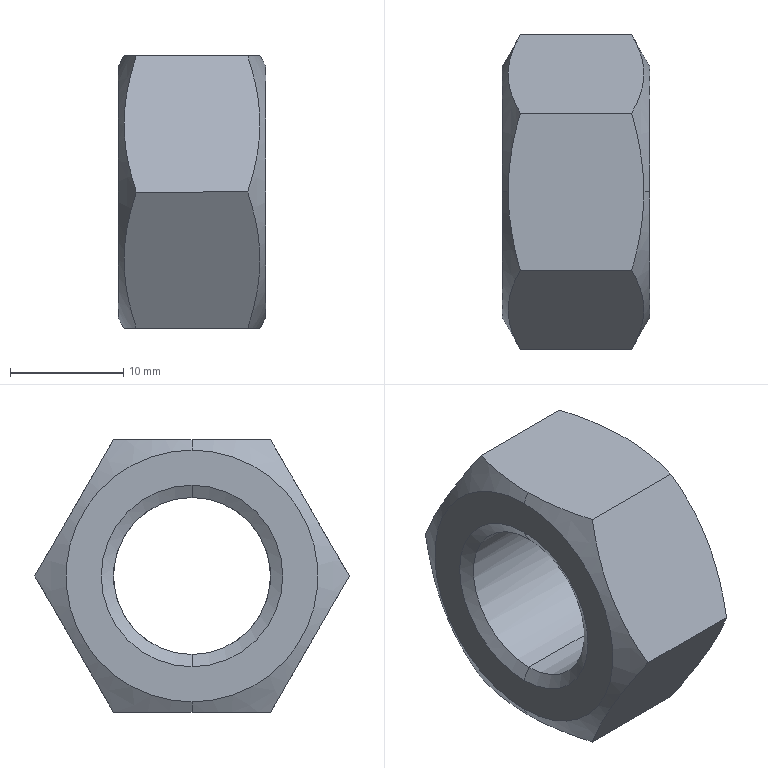Part | SolidWorks | features BaseBody 1 | 1 solid | 18 faces | box 13 x 27.713 x 24 mm | volume 4387 mm3 | cone 8 | plane 8 | cylinder 2 | commonest cylinder face diameters 13.835 x2
STEP:
#1=CARTESIAN_POINT('',(0.625,0.,6.918));
#2=VERTEX_POINT('',#1);
#3=CARTESIAN_POINT('',(0.625,0.,-6.918));
#4=VERTEX_POINT('',#3);
#5=CARTESIAN_POINT('',(0.625,0.,0.));
#6=DIRECTION('',(1.,0.,0.));
#7=DIRECTION('',(0.,0.,-1.));
#8=AXIS2_PLACEMENT_3D('',#5,#6,#7);
#9=CIRCLE('',#8,6.918);
#10=EDGE_CURVE('',#2,#4,#9,.T.);
#11=ORIENTED_EDGE('',*,*,#10,.F.);
#12=CARTESIAN_POINT('',(12.375,0.,6.918));
#13=VERTEX_POINT('',#12);
#14=CARTESIAN_POINT('',(-26.178,0.,6.918));
#15=DIRECTION('',(1.,0.,0.));
#16=VECTOR('',#15,1000.);
#17=LINE('',#14,#16);
#18=EDGE_CURVE('',#2,#13,#17,.T.);
#19=ORIENTED_EDGE('',*,*,#18,.T.);
#20=CARTESIAN_POINT('',(12.375,-6.918,0.));
#21=VERTEX_POINT('',#20);
#22=CARTESIAN_POINT('',(12.375,0.,0.));
#23=DIRECTION('',(-1.,0.,0.));
#24=DIRECTION('',(0.,0.,-1.));
#25=AXIS2_PLACEMENT_3D('',#22,#23,#24);
#26=CIRCLE('',#25,6.918);
#27=EDGE_CURVE('',#21,#13,#26,.T.);
#28=ORIENTED_EDGE('',*,*,#27,.F.);
#29=CARTESIAN_POINT('',(12.375,0.,-6.918));
#30=VERTEX_POINT('',#29);
#31=CARTESIAN_POINT('',(12.375,0.,0.));
#32=DIRECTION('',(-1.,0.,0.));
#33=DIRECTION('',(0.,0.,-1.));
#34=AXIS2_PLACEMENT_3D('',#31,#32,#33);
#35=CIRCLE('',#34,6.918);
#36=EDGE_CURVE('',#30,#21,#35,.T.);
#37=ORIENTED_EDGE('',*,*,#36,.F.);
#38=CARTESIAN_POINT('',(-26.178,0.,-6.918));
#39=DIRECTION('',(1.,0.,0.));
#40=VECTOR('',#39,1000.);
#41=LINE('',#38,#40);
#42=EDGE_CURVE('',#4,#30,#41,.T.);
#43=ORIENTED_EDGE('',*,*,#42,.F.);
#44=EDGE_LOOP('',(#11,#19,#28,#37,#43));
#45=FACE_OUTER_BOUND('',#44,.T.);
#46=CARTESIAN_POINT('',(-26.178,0.,0.));
#47=DIRECTION('',(1.,0.,0.));
#48=DIRECTION('',(0.,0.,-1.));
#49=AXIS2_PLACEMENT_3D('',#46,#47,#48);
#50=CYLINDRICAL_SURFACE('',#49,6.918);
#51=ADVANCED_FACE('',(#45),#50,.F.);
#52=ORIENTED_EDGE('',*,*,#10,.T.);
#53=CARTESIAN_POINT('',(0.,0.,-8.));
#54=VERTEX_POINT('',#53);
#55=CARTESIAN_POINT('',(0.,0.,-8.));
#56=DIRECTION('',(-0.5,0.,-0.866));
#57=VECTOR('',#56,1000.);
#58=LINE('',#55,#57);
#59=EDGE_CURVE('',#4,#54,#58,.T.);
#60=ORIENTED_EDGE('',*,*,#59,.T.);
#61=CARTESIAN_POINT('',(0.,0.,8.));
#62=VERTEX_POINT('',#61);
#63=CARTESIAN_POINT('',(0.,0.,0.));
#64=DIRECTION('',(1.,0.,0.));
#65=DIRECTION('',(0.,0.,1.));
#66=AXIS2_PLACEMENT_3D('',#63,#64,#65);
#67=CIRCLE('',#66,8.);
#68=EDGE_CURVE('',#62,#54,#67,.T.);
#69=ORIENTED_EDGE('',*,*,#68,.F.);
#70=CARTESIAN_POINT('',(0.,0.,8.));
#71=DIRECTION('',(-0.5,0.,0.866));
#72=VECTOR('',#71,1000.);
#73=LINE('',#70,#72);
#74=EDGE_CURVE('',#2,#62,#73,.T.);
#75=ORIENTED_EDGE('',*,*,#74,.F.);
#76=EDGE_LOOP('',(#52,#60,#69,#75));
#77=FACE_OUTER_BOUND('',#76,.T.);
#78=CARTESIAN_POINT('',(0.,0.,0.));
#79=DIRECTION('',(-1.,0.,0.));
#80=DIRECTION('',(0.,0.,1.));
#81=AXIS2_PLACEMENT_3D('',#78,#79,#80);
#82=CONICAL_SURFACE('',#81,8.,1.047);
#83=ADVANCED_FACE('',(#77),#82,.F.);
#84=CARTESIAN_POINT('',(12.375,6.918,0.));
#85=VERTEX_POINT('',#84);
#86=CARTESIAN_POINT('',(12.375,0.,0.));
#87=DIRECTION('',(-1.,0.,0.));
#88=DIRECTION('',(0.,0.,-1.));
#89=AXIS2_PLACEMENT_3D('',#86,#87,#88);
#90=CIRCLE('',#89,6.918);
#91=EDGE_CURVE('',#85,#30,#90,.T.);
#92=ORIENTED_EDGE('',*,*,#91,.T.);
#93=ORIENTED_EDGE('',*,*,#36,.T.);
#94=CARTESIAN_POINT('',(13.,-8.,0.));
#95=VERTEX_POINT('',#94);
#96=CARTESIAN_POINT('',(13.,-8.,0.));
#97=DIRECTION('',(0.5,-0.866,0.));
#98=VECTOR('',#97,1000.);
#99=LINE('',#96,#98);
#100=EDGE_CURVE('',#21,#95,#99,.T.);
#101=ORIENTED_EDGE('',*,*,#100,.T.);
#102=CARTESIAN_POINT('',(13.,8.,0.));
#103=VERTEX_POINT('',#102);
#104=CARTESIAN_POINT('',(13.,0.,0.));
#105=DIRECTION('',(-1.,0.,0.));
#106=DIRECTION('',(0.,1.,0.));
#107=AXIS2_PLACEMENT_3D('',#104,#105,#106);
#108=CIRCLE('',#107,8.);
#109=EDGE_CURVE('',#103,#95,#108,.T.);
#110=ORIENTED_EDGE('',*,*,#109,.F.);
#111=CARTESIAN_POINT('',(13.,8.,0.));
#112=DIRECTION('',(0.5,0.866,0.));
#113=VECTOR('',#112,1000.);
#114=LINE('',#111,#113);
#115=EDGE_CURVE('',#85,#103,#114,.T.);
#116=ORIENTED_EDGE('',*,*,#115,.F.);
#117=EDGE_LOOP('',(#92,#93,#101,#110,#116));
#118=FACE_OUTER_BOUND('',#117,.T.);
#119=CARTESIAN_POINT('',(13.,0.,0.));
#120=DIRECTION('',(1.,0.,0.));
#121=DIRECTION('',(0.,1.,0.));
#122=AXIS2_PLACEMENT_3D('',#119,#120,#121);
#123=CONICAL_SURFACE('',#122,8.,1.047);
#124=ADVANCED_FACE('',(#118),#123,.F.);
#125=CARTESIAN_POINT('',(0.,0.,-11.1));
#126=VERTEX_POINT('',#125);
#127=CARTESIAN_POINT('',(0.,0.,11.1));
#128=VERTEX_POINT('',#127);
#129=CARTESIAN_POINT('',(0.,0.,0.));
#130=DIRECTION('',(1.,0.,0.));
#131=DIRECTION('',(0.,0.,-1.));
#132=AXIS2_PLACEMENT_3D('',#129,#130,#131);
#133=CIRCLE('',#132,11.1);
#134=EDGE_CURVE('',#126,#128,#133,.T.);
#135=ORIENTED_EDGE('',*,*,#134,.T.);
#136=CARTESIAN_POINT('',(0.5196,0.,12.));
#137=VERTEX_POINT('',#136);
#138=CARTESIAN_POINT('',(1.601,0.,13.873));
#139=DIRECTION('',(0.5,0.,0.866));
#140=VECTOR('',#139,1000.);
#141=LINE('',#138,#140);
#142=EDGE_CURVE('',#128,#137,#141,.T.);
#143=ORIENTED_EDGE('',*,*,#142,.T.);
#144=CARTESIAN_POINT('',(1.591,6.928,12.));
#145=VERTEX_POINT('',#144);
#146=CARTESIAN_POINT('',(0.5196,0.,12.));
#147=CARTESIAN_POINT('',(0.5196,0.588,12.));
#148=CARTESIAN_POINT('',(0.5449,1.179,12.));
#149=CARTESIAN_POINT('',(0.643,2.347,12.));
#150=CARTESIAN_POINT('',(0.7156,2.927,12.));
#151=CARTESIAN_POINT('',(0.9956,4.658,12.));
#152=CARTESIAN_POINT('',(1.265,5.798,12.));
#153=CARTESIAN_POINT('',(1.591,6.928,12.));
#154=B_SPLINE_CURVE_WITH_KNOTS('',3,(#146,#147,#148,#149,#150,#151,#152,#153),.UNSPECIFIED.,.F.,.F.,(4,2,2,4),(0.00701,0.008756,0.0105,0.01399),.UNSPECIFIED.);
#155=EDGE_CURVE('',#137,#145,#154,.T.);
#156=ORIENTED_EDGE('',*,*,#155,.T.);
#157=CARTESIAN_POINT('',(1.591,13.856,0.000000037));
#158=VERTEX_POINT('',#157);
#159=CARTESIAN_POINT('',(1.591,6.928,12.));
#160=CARTESIAN_POINT('',(1.265,7.494,11.02));
#161=CARTESIAN_POINT('',(0.9957,8.064,10.033));
#162=CARTESIAN_POINT('',(0.6228,9.215,8.039));
#163=CARTESIAN_POINT('',(0.5204,9.797,7.032));
#164=CARTESIAN_POINT('',(0.5192,10.68,5.501));
#165=CARTESIAN_POINT('',(0.5443,10.976,4.989));
#166=CARTESIAN_POINT('',(0.642,11.561,3.975));
#167=CARTESIAN_POINT('',(0.7145,11.852,3.472));
#168=CARTESIAN_POINT('',(0.9946,12.719,1.97));
#169=CARTESIAN_POINT('',(1.264,13.29,0.9809));
#170=CARTESIAN_POINT('',(1.591,13.856,0.000000037));
#171=B_SPLINE_CURVE_WITH_KNOTS('',3,(#159,#160,#161,#162,#163,#164,#165,#166,#167,#168,#169,#170),.UNSPECIFIED.,.F.,.F.,(4,2,2,2,2,4),(0.,0.003499,0.006997,0.008746,0.0105,0.01399),.UNSPECIFIED.);
#172=EDGE_CURVE('',#145,#158,#171,.T.);
#173=ORIENTED_EDGE('',*,*,#172,.T.);
#174=CARTESIAN_POINT('',(1.591,6.928,-12.));
#175=VERTEX_POINT('',#174);
#176=CARTESIAN_POINT('',(1.591,13.856,0.000000037));
#177=CARTESIAN_POINT('',(1.265,13.291,-0.9797));
#178=CARTESIAN_POINT('',(0.9957,12.721,-1.967));
#179=CARTESIAN_POINT('',(0.6228,11.57,-3.961));
#180=CARTESIAN_POINT('',(0.5204,10.988,-4.968));
#181=CARTESIAN_POINT('',(0.5192,10.104,-6.499));
#182=CARTESIAN_POINT('',(0.5443,9.809,-7.011));
#183=CARTESIAN_POINT('',(0.642,9.223,-8.025));
#184=CARTESIAN_POINT('',(0.7145,8.933,-8.528));
#185=CARTESIAN_POINT('',(0.9946,8.066,-10.03));
#186=CARTESIAN_POINT('',(1.264,7.495,-11.019));
#187=CARTESIAN_POINT('',(1.591,6.928,-12.));
#188=B_SPLINE_CURVE_WITH_KNOTS('',3,(#176,#177,#178,#179,#180,#181,#182,#183,#184,#185,#186,#187),.UNSPECIFIED.,.F.,.F.,(4,2,2,2,2,4),(0.,0.003499,0.006997,0.008746,0.0105,0.01399),.UNSPECIFIED.);
#189=EDGE_CURVE('',#158,#175,#188,.T.);
#190=ORIENTED_EDGE('',*,*,#189,.T.);
#191=CARTESIAN_POINT('',(0.5196,0.,-12.));
#192=VERTEX_POINT('',#191);
#193=CARTESIAN_POINT('',(1.591,6.928,-12.));
#194=CARTESIAN_POINT('',(1.264,5.795,-12.));
#195=CARTESIAN_POINT('',(0.9947,4.653,-12.));
#196=CARTESIAN_POINT('',(0.6218,2.346,-12.));
#197=CARTESIAN_POINT('',(0.5196,1.18,-12.));
#198=CARTESIAN_POINT('',(0.5196,0.,-12.));
#199=B_SPLINE_CURVE_WITH_KNOTS('',3,(#193,#194,#195,#196,#197,#198),.UNSPECIFIED.,.F.,.F.,(4,2,4),(0.,0.003505,0.00701),.UNSPECIFIED.);
#200=EDGE_CURVE('',#175,#192,#199,.T.);
#201=ORIENTED_EDGE('',*,*,#200,.T.);
#202=CARTESIAN_POINT('',(1.601,0.,-13.873));
#203=DIRECTION('',(0.5,0.,-0.866));
#204=VECTOR('',#203,1000.);
#205=LINE('',#202,#204);
#206=EDGE_CURVE('',#126,#192,#205,.T.);
#207=ORIENTED_EDGE('',*,*,#206,.F.);
#208=EDGE_LOOP('',(#135,#143,#156,#173,#190,#201,#207));
#209=FACE_OUTER_BOUND('',#208,.T.);
#210=CARTESIAN_POINT('',(1.601,0.,0.));
#211=DIRECTION('',(1.,0.,0.));
#212=DIRECTION('',(0.,0.,-1.));
#213=AXIS2_PLACEMENT_3D('',#210,#211,#212);
#214=CONICAL_SURFACE('',#213,13.873,1.047);
#215=ADVANCED_FACE('',(#209),#214,.T.);
#216=CARTESIAN_POINT('',(13.,0.,-11.1));
#217=VERTEX_POINT('',#216);
#218=CARTESIAN_POINT('',(13.,0.,11.1));
#219=VERTEX_POINT('',#218);
#220=CARTESIAN_POINT('',(13.,0.,0.));
#221=DIRECTION('',(1.,0.,0.));
#222=DIRECTION('',(0.,0.,1.));
#223=AXIS2_PLACEMENT_3D('',#220,#221,#222);
#224=CIRCLE('',#223,11.1);
#225=EDGE_CURVE('',#217,#219,#224,.T.);
#226=ORIENTED_EDGE('',*,*,#225,.F.);
#227=CARTESIAN_POINT('',(12.48,0.,-12.));
#228=VERTEX_POINT('',#227);
#229=CARTESIAN_POINT('',(11.399,0.,-13.873));
#230=DIRECTION('',(-0.5,0.,-0.866));
#231=VECTOR('',#230,1000.);
#232=LINE('',#229,#231);
#233=EDGE_CURVE('',#217,#228,#232,.T.);
#234=ORIENTED_EDGE('',*,*,#233,.T.);
#235=CARTESIAN_POINT('',(11.409,6.928,-12.));
#236=VERTEX_POINT('',#235);
#237=CARTESIAN_POINT('',(12.48,0.,-12.));
#238=CARTESIAN_POINT('',(12.48,0.588,-12.));
#239=CARTESIAN_POINT('',(12.455,1.179,-12.));
#240=CARTESIAN_POINT('',(12.357,2.347,-12.));
#241=CARTESIAN_POINT('',(12.284,2.927,-12.));
#242=CARTESIAN_POINT('',(12.004,4.658,-12.));
#243=CARTESIAN_POINT('',(11.735,5.798,-12.));
#244=CARTESIAN_POINT('',(11.409,6.928,-12.));
#245=B_SPLINE_CURVE_WITH_KNOTS('',3,(#237,#238,#239,#240,#241,#242,#243,#244),.UNSPECIFIED.,.F.,.F.,(4,2,2,4),(0.00701,0.008756,0.0105,0.01399),.UNSPECIFIED.);
#246=EDGE_CURVE('',#228,#236,#245,.T.);
#247=ORIENTED_EDGE('',*,*,#246,.T.);
#248=CARTESIAN_POINT('',(11.409,13.856,0.000000014));
#249=VERTEX_POINT('',#248);
#250=CARTESIAN_POINT('',(11.409,6.928,-12.));
#251=CARTESIAN_POINT('',(11.735,7.494,-11.02));
#252=CARTESIAN_POINT('',(12.004,8.064,-10.033));
#253=CARTESIAN_POINT('',(12.377,9.215,-8.039));
#254=CARTESIAN_POINT('',(12.48,9.797,-7.032));
#255=CARTESIAN_POINT('',(12.481,10.68,-5.501));
#256=CARTESIAN_POINT('',(12.456,10.976,-4.989));
#257=CARTESIAN_POINT('',(12.358,11.561,-3.975));
#258=CARTESIAN_POINT('',(12.285,11.852,-3.472));
#259=CARTESIAN_POINT('',(12.005,12.719,-1.97));
#260=CARTESIAN_POINT('',(11.736,13.29,-0.9809));
#261=CARTESIAN_POINT('',(11.409,13.856,0.000000014));
#262=B_SPLINE_CURVE_WITH_KNOTS('',3,(#250,#251,#252,#253,#254,#255,#256,#257,#258,#259,#260,#261),.UNSPECIFIED.,.F.,.F.,(4,2,2,2,2,4),(0.,0.003499,0.006997,0.008746,0.0105,0.01399),.UNSPECIFIED.);
#263=EDGE_CURVE('',#236,#249,#262,.T.);
#264=ORIENTED_EDGE('',*,*,#263,.T.);
#265=CARTESIAN_POINT('',(11.409,6.928,12.));
#266=VERTEX_POINT('',#265);
#267=CARTESIAN_POINT('',(11.409,13.856,0.000000014));
#268=CARTESIAN_POINT('',(11.735,13.291,0.9797));
#269=CARTESIAN_POINT('',(12.004,12.721,1.967));
#270=CARTESIAN_POINT('',(12.377,11.57,3.961));
#271=CARTESIAN_POINT('',(12.48,10.988,4.968));
#272=CARTESIAN_POINT('',(12.481,10.104,6.499));
#273=CARTESIAN_POINT('',(12.456,9.809,7.011));
#274=CARTESIAN_POINT('',(12.358,9.223,8.025));
#275=CARTESIAN_POINT('',(12.285,8.933,8.528));
#276=CARTESIAN_POINT('',(12.005,8.066,10.03));
#277=CARTESIAN_POINT('',(11.736,7.495,11.019));
#278=CARTESIAN_POINT('',(11.409,6.928,12.));
#279=B_SPLINE_CURVE_WITH_KNOTS('',3,(#267,#268,#269,#270,#271,#272,#273,#274,#275,#276,#277,#278),.UNSPECIFIED.,.F.,.F.,(4,2,2,2,2,4),(0.,0.003499,0.006997,0.008746,0.0105,0.01399),.UNSPECIFIED.);
#280=EDGE_CURVE('',#249,#266,#279,.T.);
#281=ORIENTED_EDGE('',*,*,#280,.T.);
#282=CARTESIAN_POINT('',(12.48,0.,12.));
#283=VERTEX_POINT('',#282);
#284=CARTESIAN_POINT('',(11.409,6.928,12.));
#285=CARTESIAN_POINT('',(11.736,5.795,12.));
#286=CARTESIAN_POINT('',(12.005,4.653,12.));
#287=CARTESIAN_POINT('',(12.378,2.346,12.));
#288=CARTESIAN_POINT('',(12.48,1.18,12.));
#289=CARTESIAN_POINT('',(12.48,0.,12.));
#290=B_SPLINE_CURVE_WITH_KNOTS('',3,(#284,#285,#286,#287,#288,#289),.UNSPECIFIED.,.F.,.F.,(4,2,4),(0.,0.003505,0.00701),.UNSPECIFIED.);
#291=EDGE_CURVE('',#266,#283,#290,.T.);
#292=ORIENTED_EDGE('',*,*,#291,.T.);
#293=CARTESIAN_POINT('',(11.399,0.,13.873));
#294=DIRECTION('',(-0.5,0.,0.866));
#295=VECTOR('',#294,1000.);
#296=LINE('',#293,#295);
#297=EDGE_CURVE('',#219,#283,#296,.T.);
#298=ORIENTED_EDGE('',*,*,#297,.F.);
#299=EDGE_LOOP('',(#226,#234,#247,#264,#281,#292,#298));
#300=FACE_OUTER_BOUND('',#299,.T.);
#301=CARTESIAN_POINT('',(11.399,0.,0.));
#302=DIRECTION('',(-1.,0.,0.));
#303=DIRECTION('',(0.,0.,1.));
#304=AXIS2_PLACEMENT_3D('',#301,#302,#303);
#305=CONICAL_SURFACE('',#304,13.873,1.047);
#306=ADVANCED_FACE('',(#300),#305,.T.);
#307=ORIENTED_EDGE('',*,*,#18,.F.);
#308=CARTESIAN_POINT('',(0.625,0.,0.));
#309=DIRECTION('',(1.,0.,0.));
#310=DIRECTION('',(0.,0.,-1.));
#311=AXIS2_PLACEMENT_3D('',#308,#309,#310);
#312=CIRCLE('',#311,6.918);
#313=EDGE_CURVE('',#4,#2,#312,.T.);
#314=ORIENTED_EDGE('',*,*,#313,.F.);
#315=ORIENTED_EDGE('',*,*,#42,.T.);
#316=ORIENTED_EDGE('',*,*,#91,.F.);
#317=CARTESIAN_POINT('',(12.375,0.,0.));
#318=DIRECTION('',(-1.,0.,0.));
#319=DIRECTION('',(0.,0.,-1.));
#320=AXIS2_PLACEMENT_3D('',#317,#318,#319);
#321=CIRCLE('',#320,6.918);
#322=EDGE_CURVE('',#13,#85,#321,.T.);
#323=ORIENTED_EDGE('',*,*,#322,.F.);
#324=EDGE_LOOP('',(#307,#314,#315,#316,#323));
#325=FACE_OUTER_BOUND('',#324,.T.);
#326=CARTESIAN_POINT('',(-26.178,0.,0.));
#327=DIRECTION('',(1.,0.,0.));
#328=DIRECTION('',(0.,0.,-1.));
#329=AXIS2_PLACEMENT_3D('',#326,#327,#328);
#330=CYLINDRICAL_SURFACE('',#329,6.918);
#331=ADVANCED_FACE('',(#325),#330,.F.);
#332=ORIENTED_EDGE('',*,*,#59,.F.);
#333=ORIENTED_EDGE('',*,*,#313,.T.);
#334=ORIENTED_EDGE('',*,*,#74,.T.);
#335=CARTESIAN_POINT('',(0.,0.,0.));
#336=DIRECTION('',(1.,0.,0.));
#337=DIRECTION('',(0.,0.,1.));
#338=AXIS2_PLACEMENT_3D('',#335,#336,#337);
#339=CIRCLE('',#338,8.);
#340=EDGE_CURVE('',#54,#62,#339,.T.);
#341=ORIENTED_EDGE('',*,*,#340,.F.);
#342=EDGE_LOOP('',(#332,#333,#334,#341));
#343=FACE_OUTER_BOUND('',#342,.T.);
#344=CARTESIAN_POINT('',(0.,0.,0.));
#345=DIRECTION('',(-1.,0.,0.));
#346=DIRECTION('',(0.,0.,1.));
#347=AXIS2_PLACEMENT_3D('',#344,#345,#346);
#348=CONICAL_SURFACE('',#347,8.,1.047);
#349=ADVANCED_FACE('',(#343),#348,.F.);
#350=ORIENTED_EDGE('',*,*,#100,.F.);
#351=ORIENTED_EDGE('',*,*,#27,.T.);
#352=ORIENTED_EDGE('',*,*,#322,.T.);
#353=ORIENTED_EDGE('',*,*,#115,.T.);
#354=CARTESIAN_POINT('',(13.,0.,0.));
#355=DIRECTION('',(-1.,0.,0.));
#356=DIRECTION('',(0.,1.,0.));
#357=AXIS2_PLACEMENT_3D('',#354,#355,#356);
#358=CIRCLE('',#357,8.);
#359=EDGE_CURVE('',#95,#103,#358,.T.);
#360=ORIENTED_EDGE('',*,*,#359,.F.);
#361=EDGE_LOOP('',(#350,#351,#352,#353,#360));
#362=FACE_OUTER_BOUND('',#361,.T.);
#363=CARTESIAN_POINT('',(13.,0.,0.));
#364=DIRECTION('',(1.,0.,0.));
#365=DIRECTION('',(0.,1.,0.));
#366=AXIS2_PLACEMENT_3D('',#363,#364,#365);
#367=CONICAL_SURFACE('',#366,8.,1.047);
#368=ADVANCED_FACE('',(#362),#367,.F.);
#369=ORIENTED_EDGE('',*,*,#68,.T.);
#370=ORIENTED_EDGE('',*,*,#340,.T.);
#371=EDGE_LOOP('',(#369,#370));
#372=FACE_BOUND('',#371,.T.);
#373=ORIENTED_EDGE('',*,*,#134,.F.);
#374=CARTESIAN_POINT('',(0.,0.,0.));
#375=DIRECTION('',(1.,0.,0.));
#376=DIRECTION('',(0.,0.,-1.));
#377=AXIS2_PLACEMENT_3D('',#374,#375,#376);
#378=CIRCLE('',#377,11.1);
#379=EDGE_CURVE('',#128,#126,#378,.T.);
#380=ORIENTED_EDGE('',*,*,#379,.F.);
#381=EDGE_LOOP('',(#373,#380));
#382=FACE_OUTER_BOUND('',#381,.T.);
#383=CARTESIAN_POINT('',(0.,0.,0.));
#384=DIRECTION('',(1.,0.,0.));
#385=DIRECTION('',(0.,0.,-1.));
#386=AXIS2_PLACEMENT_3D('',#383,#384,#385);
#387=PLANE('',#386);
#388=ADVANCED_FACE('',(#372,#382),#387,.F.);
#389=ORIENTED_EDGE('',*,*,#109,.T.);
#390=ORIENTED_EDGE('',*,*,#359,.T.);
#391=EDGE_LOOP('',(#389,#390));
#392=FACE_BOUND('',#391,.T.);
#393=CARTESIAN_POINT('',(13.,0.,0.));
#394=DIRECTION('',(1.,0.,0.));
#395=DIRECTION('',(0.,0.,1.));
#396=AXIS2_PLACEMENT_3D('',#393,#394,#395);
#397=CIRCLE('',#396,11.1);
#398=EDGE_CURVE('',#219,#217,#397,.T.);
#399=ORIENTED_EDGE('',*,*,#398,.T.);
#400=ORIENTED_EDGE('',*,*,#225,.T.);
#401=EDGE_LOOP('',(#399,#400));
#402=FACE_OUTER_BOUND('',#401,.T.);
#403=CARTESIAN_POINT('',(13.,0.,0.));
#404=DIRECTION('',(1.,0.,0.));
#405=DIRECTION('',(0.,0.,-1.));
#406=AXIS2_PLACEMENT_3D('',#403,#404,#405);
#407=PLANE('',#406);
#408=ADVANCED_FACE('',(#392,#402),#407,.T.);
#409=ORIENTED_EDGE('',*,*,#142,.F.);
#410=ORIENTED_EDGE('',*,*,#379,.T.);
#411=ORIENTED_EDGE('',*,*,#206,.T.);
#412=CARTESIAN_POINT('',(1.591,-6.928,-12.));
#413=VERTEX_POINT('',#412);
#414=CARTESIAN_POINT('',(0.5196,0.,-12.));
#415=CARTESIAN_POINT('',(0.5196,-0.588,-12.));
#416=CARTESIAN_POINT('',(0.5449,-1.179,-12.));
#417=CARTESIAN_POINT('',(0.643,-2.347,-12.));
#418=CARTESIAN_POINT('',(0.7156,-2.927,-12.));
#419=CARTESIAN_POINT('',(0.9956,-4.658,-12.));
#420=CARTESIAN_POINT('',(1.265,-5.798,-12.));
#421=CARTESIAN_POINT('',(1.591,-6.928,-12.));
#422=B_SPLINE_CURVE_WITH_KNOTS('',3,(#414,#415,#416,#417,#418,#419,#420,#421),.UNSPECIFIED.,.F.,.F.,(4,2,2,4),(0.00701,0.008756,0.0105,0.01399),.UNSPECIFIED.);
#423=EDGE_CURVE('',#192,#413,#422,.T.);
#424=ORIENTED_EDGE('',*,*,#423,.T.);
#425=CARTESIAN_POINT('',(1.591,-13.856,-0.000000037));
#426=VERTEX_POINT('',#425);
#427=CARTESIAN_POINT('',(1.591,-6.928,-12.));
#428=CARTESIAN_POINT('',(1.265,-7.494,-11.02));
#429=CARTESIAN_POINT('',(0.9957,-8.064,-10.033));
#430=CARTESIAN_POINT('',(0.6228,-9.215,-8.039));
#431=CARTESIAN_POINT('',(0.5204,-9.797,-7.032));
#432=CARTESIAN_POINT('',(0.5192,-10.68,-5.501));
#433=CARTESIAN_POINT('',(0.5443,-10.976,-4.989));
#434=CARTESIAN_POINT('',(0.642,-11.561,-3.975));
#435=CARTESIAN_POINT('',(0.7145,-11.852,-3.472));
#436=CARTESIAN_POINT('',(0.9946,-12.719,-1.97));
#437=CARTESIAN_POINT('',(1.264,-13.29,-0.9809));
#438=CARTESIAN_POINT('',(1.591,-13.856,-0.000000037));
#439=B_SPLINE_CURVE_WITH_KNOTS('',3,(#427,#428,#429,#430,#431,#432,#433,#434,#435,#436,#437,#438),.UNSPECIFIED.,.F.,.F.,(4,2,2,2,2,4),(0.,0.003499,0.006997,0.008746,0.0105,0.01399),.UNSPECIFIED.);
#440=EDGE_CURVE('',#413,#426,#439,.T.);
#441=ORIENTED_EDGE('',*,*,#440,.T.);
#442=CARTESIAN_POINT('',(1.591,-6.928,12.));
#443=VERTEX_POINT('',#442);
#444=CARTESIAN_POINT('',(1.591,-13.856,-0.000000037));
#445=CARTESIAN_POINT('',(1.265,-13.291,0.9797));
#446=CARTESIAN_POINT('',(0.9957,-12.721,1.967));
#447=CARTESIAN_POINT('',(0.6228,-11.57,3.961));
#448=CARTESIAN_POINT('',(0.5204,-10.988,4.968));
#449=CARTESIAN_POINT('',(0.5192,-10.104,6.499));
#450=CARTESIAN_POINT('',(0.5443,-9.809,7.011));
#451=CARTESIAN_POINT('',(0.642,-9.223,8.025));
#452=CARTESIAN_POINT('',(0.7145,-8.933,8.528));
#453=CARTESIAN_POINT('',(0.9946,-8.066,10.03));
#454=CARTESIAN_POINT('',(1.264,-7.495,11.019));
#455=CARTESIAN_POINT('',(1.591,-6.928,12.));
#456=B_SPLINE_CURVE_WITH_KNOTS('',3,(#444,#445,#446,#447,#448,#449,#450,#451,#452,#453,#454,#455),.UNSPECIFIED.,.F.,.F.,(4,2,2,2,2,4),(0.,0.003499,0.006997,0.008746,0.0105,0.01399),.UNSPECIFIED.);
#457=EDGE_CURVE('',#426,#443,#456,.T.);
#458=ORIENTED_EDGE('',*,*,#457,.T.);
#459=CARTESIAN_POINT('',(1.591,-6.928,12.));
#460=CARTESIAN_POINT('',(1.264,-5.795,12.));
#461=CARTESIAN_POINT('',(0.9947,-4.653,12.));
#462=CARTESIAN_POINT('',(0.6218,-2.346,12.));
#463=CARTESIAN_POINT('',(0.5196,-1.18,12.));
#464=CARTESIAN_POINT('',(0.5196,0.,12.));
#465=B_SPLINE_CURVE_WITH_KNOTS('',3,(#459,#460,#461,#462,#463,#464),.UNSPECIFIED.,.F.,.F.,(4,2,4),(0.,0.003505,0.00701),.UNSPECIFIED.);
#466=EDGE_CURVE('',#443,#137,#465,.T.);
#467=ORIENTED_EDGE('',*,*,#466,.T.);
#468=EDGE_LOOP('',(#409,#410,#411,#424,#441,#458,#467));
#469=FACE_OUTER_BOUND('',#468,.T.);
#470=CARTESIAN_POINT('',(1.601,0.,0.));
#471=DIRECTION('',(1.,0.,0.));
#472=DIRECTION('',(0.,0.,-1.));
#473=AXIS2_PLACEMENT_3D('',#470,#471,#472);
#474=CONICAL_SURFACE('',#473,13.873,1.047);
#475=ADVANCED_FACE('',(#469),#474,.T.);
#476=ORIENTED_EDGE('',*,*,#233,.F.);
#477=ORIENTED_EDGE('',*,*,#398,.F.);
#478=ORIENTED_EDGE('',*,*,#297,.T.);
#479=CARTESIAN_POINT('',(11.409,-6.928,12.));
#480=VERTEX_POINT('',#479);
#481=CARTESIAN_POINT('',(12.48,0.,12.));
#482=CARTESIAN_POINT('',(12.48,-0.588,12.));
#483=CARTESIAN_POINT('',(12.455,-1.179,12.));
#484=CARTESIAN_POINT('',(12.357,-2.347,12.));
#485=CARTESIAN_POINT('',(12.284,-2.927,12.));
#486=CARTESIAN_POINT('',(12.004,-4.658,12.));
#487=CARTESIAN_POINT('',(11.735,-5.798,12.));
#488=CARTESIAN_POINT('',(11.409,-6.928,12.));
#489=B_SPLINE_CURVE_WITH_KNOTS('',3,(#481,#482,#483,#484,#485,#486,#487,#488),.UNSPECIFIED.,.F.,.F.,(4,2,2,4),(0.00701,0.008756,0.0105,0.01399),.UNSPECIFIED.);
#490=EDGE_CURVE('',#283,#480,#489,.T.);
#491=ORIENTED_EDGE('',*,*,#490,.T.);
#492=CARTESIAN_POINT('',(11.409,-13.856,0.000000037));
#493=VERTEX_POINT('',#492);
#494=CARTESIAN_POINT('',(11.409,-6.928,12.));
#495=CARTESIAN_POINT('',(11.735,-7.494,11.02));
#496=CARTESIAN_POINT('',(12.004,-8.064,10.033));
#497=CARTESIAN_POINT('',(12.377,-9.215,8.039));
#498=CARTESIAN_POINT('',(12.48,-9.797,7.032));
#499=CARTESIAN_POINT('',(12.481,-10.68,5.501));
#500=CARTESIAN_POINT('',(12.456,-10.976,4.989));
#501=CARTESIAN_POINT('',(12.358,-11.561,3.975));
#502=CARTESIAN_POINT('',(12.285,-11.852,3.472));
#503=CARTESIAN_POINT('',(12.005,-12.719,1.97));
#504=CARTESIAN_POINT('',(11.736,-13.29,0.9809));
#505=CARTESIAN_POINT('',(11.409,-13.856,0.000000037));
#506=B_SPLINE_CURVE_WITH_KNOTS('',3,(#494,#495,#496,#497,#498,#499,#500,#501,#502,#503,#504,#505),.UNSPECIFIED.,.F.,.F.,(4,2,2,2,2,4),(0.,0.003499,0.006997,0.008746,0.0105,0.01399),.UNSPECIFIED.);
#507=EDGE_CURVE('',#480,#493,#506,.T.);
#508=ORIENTED_EDGE('',*,*,#507,.T.);
#509=CARTESIAN_POINT('',(11.409,-6.928,-12.));
#510=VERTEX_POINT('',#509);
#511=CARTESIAN_POINT('',(11.409,-13.856,0.000000037));
#512=CARTESIAN_POINT('',(11.735,-13.291,-0.9797));
#513=CARTESIAN_POINT('',(12.004,-12.721,-1.967));
#514=CARTESIAN_POINT('',(12.377,-11.57,-3.961));
#515=CARTESIAN_POINT('',(12.48,-10.988,-4.968));
#516=CARTESIAN_POINT('',(12.481,-10.104,-6.499));
#517=CARTESIAN_POINT('',(12.456,-9.809,-7.011));
#518=CARTESIAN_POINT('',(12.358,-9.223,-8.025));
#519=CARTESIAN_POINT('',(12.285,-8.933,-8.528));
#520=CARTESIAN_POINT('',(12.005,-8.066,-10.03));
#521=CARTESIAN_POINT('',(11.736,-7.495,-11.019));
#522=CARTESIAN_POINT('',(11.409,-6.928,-12.));
#523=B_SPLINE_CURVE_WITH_KNOTS('',3,(#511,#512,#513,#514,#515,#516,#517,#518,#519,#520,#521,#522),.UNSPECIFIED.,.F.,.F.,(4,2,2,2,2,4),(0.,0.003499,0.006997,0.008746,0.0105,0.01399),.UNSPECIFIED.);
#524=EDGE_CURVE('',#493,#510,#523,.T.);
#525=ORIENTED_EDGE('',*,*,#524,.T.);
#526=CARTESIAN_POINT('',(11.409,-6.928,-12.));
#527=CARTESIAN_POINT('',(11.736,-5.795,-12.));
#528=CARTESIAN_POINT('',(12.005,-4.653,-12.));
#529=CARTESIAN_POINT('',(12.378,-2.346,-12.));
#530=CARTESIAN_POINT('',(12.48,-1.18,-12.));
#531=CARTESIAN_POINT('',(12.48,0.,-12.));
#532=B_SPLINE_CURVE_WITH_KNOTS('',3,(#526,#527,#528,#529,#530,#531),.UNSPECIFIED.,.F.,.F.,(4,2,4),(0.,0.003505,0.00701),.UNSPECIFIED.);
#533=EDGE_CURVE('',#510,#228,#532,.T.);
#534=ORIENTED_EDGE('',*,*,#533,.T.);
#535=EDGE_LOOP('',(#476,#477,#478,#491,#508,#525,#534));
#536=FACE_OUTER_BOUND('',#535,.T.);
#537=CARTESIAN_POINT('',(11.399,0.,0.));
#538=DIRECTION('',(-1.,0.,0.));
#539=DIRECTION('',(0.,0.,1.));
#540=AXIS2_PLACEMENT_3D('',#537,#538,#539);
#541=CONICAL_SURFACE('',#540,13.873,1.047);
#542=ADVANCED_FACE('',(#536),#541,.T.);
#543=ORIENTED_EDGE('',*,*,#507,.F.);
#544=CARTESIAN_POINT('',(0.,-6.928,12.));
#545=DIRECTION('',(-1.,0.,0.));
#546=VECTOR('',#545,1000.);
#547=LINE('',#544,#546);
#548=EDGE_CURVE('',#480,#443,#547,.T.);
#549=ORIENTED_EDGE('',*,*,#548,.T.);
#550=ORIENTED_EDGE('',*,*,#457,.F.);
#551=CARTESIAN_POINT('',(0.,-13.856,0.));
#552=DIRECTION('',(1.,0.,0.));
#553=VECTOR('',#552,1000.);
#554=LINE('',#551,#553);
#555=EDGE_CURVE('',#426,#493,#554,.T.);
#556=ORIENTED_EDGE('',*,*,#555,.T.);
#557=EDGE_LOOP('',(#543,#549,#550,#556));
#558=FACE_OUTER_BOUND('',#557,.T.);
#559=CARTESIAN_POINT('',(0.,-13.856,0.));
#560=DIRECTION('',(0.,-0.866,0.5));
#561=DIRECTION('',(0.,-0.5,-0.866));
#562=AXIS2_PLACEMENT_3D('',#559,#560,#561);
#563=PLANE('',#562);
#564=ADVANCED_FACE('',(#558),#563,.T.);
#565=ORIENTED_EDGE('',*,*,#524,.F.);
#566=ORIENTED_EDGE('',*,*,#555,.F.);
#567=ORIENTED_EDGE('',*,*,#440,.F.);
#568=CARTESIAN_POINT('',(0.,-6.928,-12.));
#569=DIRECTION('',(1.,0.,0.));
#570=VECTOR('',#569,1000.);
#571=LINE('',#568,#570);
#572=EDGE_CURVE('',#413,#510,#571,.T.);
#573=ORIENTED_EDGE('',*,*,#572,.T.);
#574=EDGE_LOOP('',(#565,#566,#567,#573));
#575=FACE_OUTER_BOUND('',#574,.T.);
#576=CARTESIAN_POINT('',(0.,-6.928,-12.));
#577=DIRECTION('',(0.,-0.866,-0.5));
#578=DIRECTION('',(0.,0.5,-0.866));
#579=AXIS2_PLACEMENT_3D('',#576,#577,#578);
#580=PLANE('',#579);
#581=ADVANCED_FACE('',(#575),#580,.T.);
#582=ORIENTED_EDGE('',*,*,#533,.F.);
#583=ORIENTED_EDGE('',*,*,#572,.F.);
#584=ORIENTED_EDGE('',*,*,#423,.F.);
#585=ORIENTED_EDGE('',*,*,#200,.F.);
#586=CARTESIAN_POINT('',(0.,6.928,-12.));
#587=DIRECTION('',(1.,0.,0.));
#588=VECTOR('',#587,1000.);
#589=LINE('',#586,#588);
#590=EDGE_CURVE('',#175,#236,#589,.T.);
#591=ORIENTED_EDGE('',*,*,#590,.T.);
#592=ORIENTED_EDGE('',*,*,#246,.F.);
#593=EDGE_LOOP('',(#582,#583,#584,#585,#591,#592));
#594=FACE_OUTER_BOUND('',#593,.T.);
#595=CARTESIAN_POINT('',(0.,6.928,-12.));
#596=DIRECTION('',(0.,0.,-1.));
#597=DIRECTION('',(0.,1.,0.));
#598=AXIS2_PLACEMENT_3D('',#595,#596,#597);
#599=PLANE('',#598);
#600=ADVANCED_FACE('',(#594),#599,.T.);
#601=ORIENTED_EDGE('',*,*,#263,.F.);
#602=ORIENTED_EDGE('',*,*,#590,.F.);
#603=ORIENTED_EDGE('',*,*,#189,.F.);
#604=CARTESIAN_POINT('',(0.,13.856,0.));
#605=DIRECTION('',(1.,0.,0.));
#606=VECTOR('',#605,1000.);
#607=LINE('',#604,#606);
#608=EDGE_CURVE('',#158,#249,#607,.T.);
#609=ORIENTED_EDGE('',*,*,#608,.T.);
#610=EDGE_LOOP('',(#601,#602,#603,#609));
#611=FACE_OUTER_BOUND('',#610,.T.);
#612=CARTESIAN_POINT('',(0.,13.856,0.));
#613=DIRECTION('',(0.,0.866,-0.5));
#614=DIRECTION('',(0.,0.5,0.866));
#615=AXIS2_PLACEMENT_3D('',#612,#613,#614);
#616=PLANE('',#615);
#617=ADVANCED_FACE('',(#611),#616,.T.);
#618=ORIENTED_EDGE('',*,*,#280,.F.);
#619=ORIENTED_EDGE('',*,*,#608,.F.);
#620=ORIENTED_EDGE('',*,*,#172,.F.);
#621=CARTESIAN_POINT('',(0.,6.928,12.));
#622=DIRECTION('',(1.,0.,0.));
#623=VECTOR('',#622,1000.);
#624=LINE('',#621,#623);
#625=EDGE_CURVE('',#145,#266,#624,.T.);
#626=ORIENTED_EDGE('',*,*,#625,.T.);
#627=EDGE_LOOP('',(#618,#619,#620,#626));
#628=FACE_OUTER_BOUND('',#627,.T.);
#629=CARTESIAN_POINT('',(0.,6.928,12.));
#630=DIRECTION('',(0.,0.866,0.5));
#631=DIRECTION('',(0.,-0.5,0.866));
#632=AXIS2_PLACEMENT_3D('',#629,#630,#631);
#633=PLANE('',#632);
#634=ADVANCED_FACE('',(#628),#633,.T.);
#635=ORIENTED_EDGE('',*,*,#291,.F.);
#636=ORIENTED_EDGE('',*,*,#625,.F.);
#637=ORIENTED_EDGE('',*,*,#155,.F.);
#638=ORIENTED_EDGE('',*,*,#466,.F.);
#639=ORIENTED_EDGE('',*,*,#548,.F.);
#640=ORIENTED_EDGE('',*,*,#490,.F.);
#641=EDGE_LOOP('',(#635,#636,#637,#638,#639,#640));
#642=FACE_OUTER_BOUND('',#641,.T.);
#643=CARTESIAN_POINT('',(0.,-6.928,12.));
#644=DIRECTION('',(0.,0.,1.));
#645=DIRECTION('',(1.,0.,0.));
#646=AXIS2_PLACEMENT_3D('',#643,#644,#645);
#647=PLANE('',#646);
#648=ADVANCED_FACE('',(#642),#647,.T.);
#649=CLOSED_SHELL('',(#51,#83,#124,#215,#306,#331,#349,#368,#388,#408,#475,#542,#564,#581,#600,#617,#634,#648));
#650=MANIFOLD_SOLID_BREP('',#649);
#651=CARTESIAN_POINT('',(0.,0.,0.));
#652=DIRECTION('',(0.,0.,1.));
#653=DIRECTION('',(1.,0.,0.));
#654=AXIS2_PLACEMENT_3D('',#651,#652,#653);
#655=(LENGTH_UNIT()NAMED_UNIT(*)SI_UNIT(.MILLI.,.METRE.));
#656=UNCERTAINTY_MEASURE_WITH_UNIT(LENGTH_MEASURE(0.00001),#655,'','');
#657=(NAMED_UNIT(*)PLANE_ANGLE_UNIT()SI_UNIT($,.RADIAN.));
#658=(NAMED_UNIT(*)SI_UNIT($,.STERADIAN.)SOLID_ANGLE_UNIT());
#659=(GEOMETRIC_REPRESENTATION_CONTEXT(3)GLOBAL_UNCERTAINTY_ASSIGNED_CONTEXT((#656))GLOBAL_UNIT_ASSIGNED_CONTEXT((#655,#657,#658))REPRESENTATION_CONTEXT('',''));
#660=ADVANCED_BREP_SHAPE_REPRESENTATION('',(#650,#654),#659);